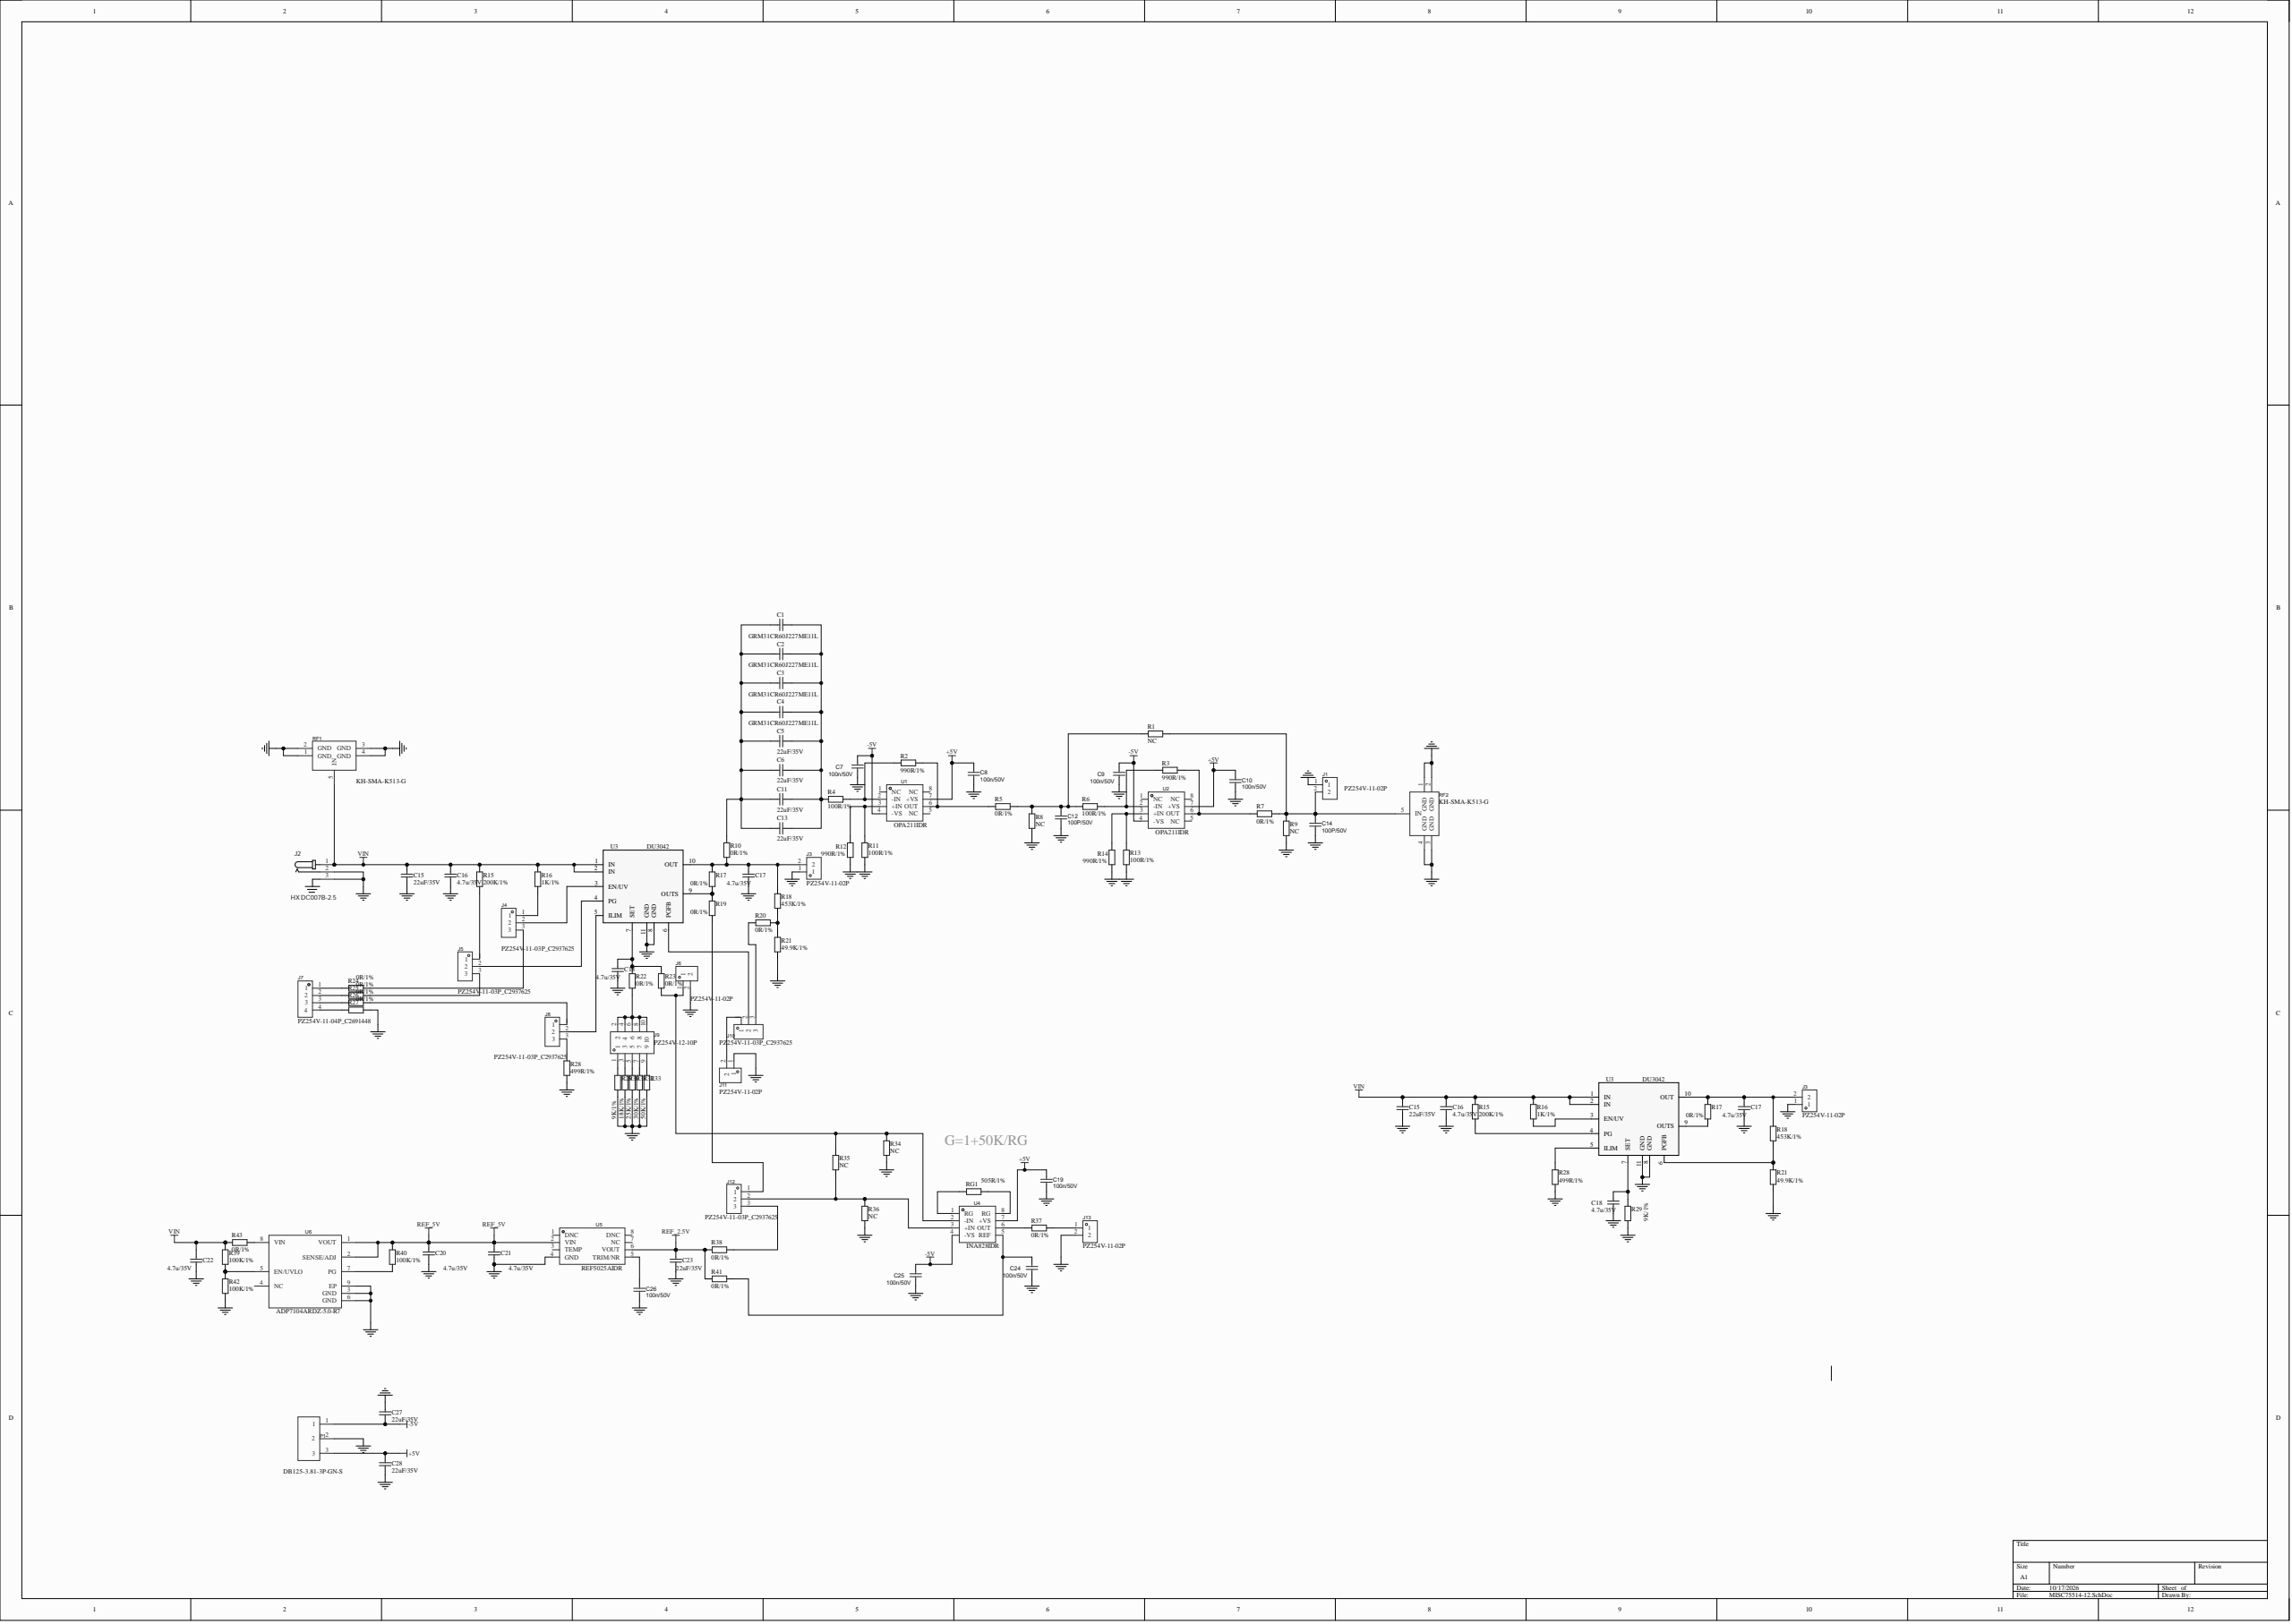Circuit board | Altium Designer | 107 parts | 62 nets
Bill of materials:
Comment,Description,Designator,Footprint,LibRef,Quantity
"GRM31CR60J227ME11L","SMD capacitor","C1, C2, C3, C4","C1206","C","4"
"22uF/35V","SMD capacitor","C5, C6, C11, C13, C15, C23, C27, C28","C1206","C","9"
"100n/50V","","C7, C8, C9, C10, C19, C24, C25, C26","C0603","1uF","8"
"100P/50V","","C12, C14","C0603","1uF","2"
"4.7u/35V","SMD capacitor","C16, C17, C18, C20, C21, C22","C0805","C","9"
"PZ254V-11-02P","","J1, J3, J6, J11, J13","HDR-TH_2P-P2.54-V-M","PZ254V-11-02P","6"
"HX DC007B-2.5","","J2","DC-IN-TH_HX-DC007B-2.5","HX DC007B-2.5","1"
"PZ254V-11-03P_C2937625","","J4, J5, J8, J10, J12","HDR-TH_3P-P2.54-V-M","PZ254V-11-03P_C2937625","5"
"PZ254V-11-04P_C2691448","","J7","HDR-TH_4P-P2.54-V-M","PZ254V-11-04P_C2691448","1"
"PZ254V-12-10P","","J9","HDR-TH_10P-P2.54-V-M-R2-C5-S2.54","PZ254V-12-10P","1"
"DB125-3.81-3P-GN-S","","P1","CONN-TH_3P-P3.81_L7.4-W11.4","WJ124-3.81-3P","1"
"NC","SMD resistor","R1, R8, R9, R34, R35, R36","R0603","R","6"
"990R/1%","SMD resistor","R2, R3, R12, R14","R0603","R","4"
"100R/1%","SMD resistor","R4, R6, R11, R13","R0603","R","4"
"0R/1%","SMD resistor","R5, R7, R10, R17, R19, R20, R22, R23, R24, R25, R26, R27, R37, R38, R41, R43","R0603","R","17"
"200K/1%","SMD resistor","R15","R0603","R","2"
"1K/1%","SMD resistor","R16","R0603","R","2"
"453K/1%","SMD resistor","R18","R0603","R","2"
"49.9K/1%","SMD resistor","R21","R0603","R","2"
"499R/1%","SMD resistor","R28","R0603","R","2"
"9K/1%","SMD resistor","R29","R0603","R","2"
"18K/1%","SMD resistor","R30","R0603","R","1"
"25K/1%","SMD resistor","R31","R0603","R","1"
"30K/1%","SMD resistor","R32","R0603","R","1"
"50K/1%","SMD resistor","R33","R0603","R","1"
"100K/1%","SMD resistor","R39, R40, R42","R0603","R","3"
"KH-SMA-K513-G","","RF1, RF2","ANT-TH_KH-SMA-K513-G","KH-SMA-K513-G","2"
"505R/1%","SMD resistor","RG1","R0603","R","1"
"OPA211IDR","","U1, U2","SOIC-8_L5.0-W4.0-P1.27-LS6.0-BL","INA828IDR","2"
"DU3042","No Description Available","U3","WSON-10_L3.0-W3.0-P0.50-BL-EP","DAC53202RTER","2"
"INA828IDR","","U4","SOIC-8_L5.0-W4.0-P1.27-LS6.0-BL","INA828IDR","1"
"REF5025AIDR","","U5","SOIC-8_L5.0-W4.0-P1.27-LS6.0-BL","REF5025AIDR","1"
"ADP7104ARDZ-5.0-R7","","U6","SOIC-8_L4.9-W3.9-P1.27-LS6.0-BL-EP","ADP7104ARDZ-5.0-R7","1"
Netlist (Protel format):
[
C1
C1206
GRM31CR60J227ME11L



]
[
C2
C1206
GRM31CR60J227ME11L



]
[
C3
C1206
GRM31CR60J227ME11L



]
[
C4
C1206
GRM31CR60J227ME11L



]
[
C5
C1206
22uF/35V



]
[
C6
C1206
22uF/35V



]
[
C7
C0603
100n/50V



]
[
C8
C0603
100n/50V



]
[
C9
C0603
100n/50V



]
[
C10
C0603
100n/50V



]
[
C11
C1206
22uF/35V



]
[
C12
C0603
100P/50V



]
[
C13
C1206
22uF/35V



]
[
C14
C0603
100P/50V



]
[
C15
C1206
22uF/35V



]
[
C15
C1206
22uF/35V



]
[
C16
C0805
4.7u/35V



]
[
C16
C0805
4.7u/35V



]
[
C17
C0805
4.7u/35V



]
[
C17
C0805
4.7u/35V



]
[
C18
C0805
4.7u/35V



]
[
C18
C0805
4.7u/35V



]
[
C19
C0603
100n/50V



]
[
C20
C0805
4.7u/35V



]
[
C21
C0805
4.7u/35V



]
[
C22
C0805
4.7u/35V



]
[
C23
C1206
22uF/35V



]
[
C24
C0603
100n/50V



]
[
C25
C0603
100n/50V



]
[
C26
C0603
100n/50V



]
[
C27
C1206
22uF/35V



]
[
C28
C1206
22uF/35V



]
[
J1
HDR-TH_2P-P2.54-V-M
PZ254V-11-02P



]
[
J2
DC-IN-TH_HX-DC007B-2.5
HX DC007B-2.5



]
[
J3
HDR-TH_2P-P2.54-V-M
PZ254V-11-02P



]
[
J3
HDR-TH_2P-P2.54-V-M
PZ254V-11-02P



]
[
J4
HDR-TH_3P-P2.54-V-M
PZ254V-11-03P_C2937625



]
[
J5
HDR-TH_3P-P2.54-V-M
PZ254V-11-03P_C2937625



]
[
J6
HDR-TH_2P-P2.54-V-M
PZ254V-11-02P



]
[
J7
HDR-TH_4P-P2.54-V-M
PZ254V-11-04P_C2691448



]
[
J8
HDR-TH_3P-P2.54-V-M
PZ254V-11-03P_C2937625



]
[
J9
HDR-TH_10P-P2.54-V-M-R2-C5-S2.54
PZ254V-12-10P



]
[
J10
HDR-TH_3P-P2.54-V-M
PZ254V-11-03P_C2937625



]
[
J11
HDR-TH_2P-P2.54-V-M
PZ254V-11-02P



]
[
J12
HDR-TH_3P-P2.54-V-M
PZ254V-11-03P_C2937625



]
[
J13
HDR-TH_2P-P2.54-V-M
PZ254V-11-02P



]
[
P1
CONN-TH_3P-P3.81_L7.4-W11.4
DB125-3.81-3P-GN-S



]
[
R1
R0603
NC



]
[
R2
R0603
990R/1%



]
[
R3
R0603
990R/1%



]
[
R4
R0603
100R/1%



]
[
R5
R0603
0R/1%



]
[
R6
R0603
100R/1%



]
[
R7
R0603
0R/1%



]
[
R8
R0603
NC



]
[
R9
R0603
NC



]
[
R10
R0603
0R/1%



]
[
R11
R0603
100R/1%



]
[
R12
R0603
990R/1%



]
[
R13
R0603
100R/1%



]
[
R14
R0603
990R/1%



]
[
R15
R0603
200K/1%



]
[
R15
R0603
200K/1%



]
[
R16
R0603
1K/1%



]
[
R16
R0603
1K/1%



]
[
R17
R0603
0R/1%



]
[
R17
R0603
0R/1%



]
[
R18
R0603
453K/1%



]
[
R18
R0603
453K/1%



]
[
R19
R0603
0R/1%



]
[
R20
R0603
0R/1%



]
[
R21
R0603
49.9K/1%



]
[
R21
R0603
49.9K/1%



]
[
R22
R0603
0R/1%



]
[
R23
R0603
0R/1%



]
[
R24
R0603
0R/1%



]
[
R25
R0603
0R/1%



]
[
R26
R0603
0R/1%



]
[
R27
R0603
0R/1%



]
[
R28
R0603
499R/1%



]
[
R28
R0603
499R/1%



]
[
R29
R0603
9K/1%



]
[
R29
R0603
9K/1%



]
[
R30
R0603
18K/1%



]
[
R31
R0603
25K/1%



]
[
R32
R0603
30K/1%



]
[
R33
R0603
50K/1%



]
[
R34
R0603
NC



]
[
R35
R0603
NC



]
[
R36
R0603
NC



]
[
R37
R0603
0R/1%



]
[
R38
R0603
0R/1%



]
[
R39
R0603
100K/1%



]
[
R40
R0603
100K/1%



]
[
R41
R0603
0R/1%



]
[
R42
R0603
100K/1%



]
[
R43
R0603
0R/1%



]
[
RF1
ANT-TH_KH-SMA-K513-G
KH-SMA-K513-G



]
[
RF2
ANT-TH_KH-SMA-K513-G
KH-SMA-K513-G



]
[
RG1
R0603
505R/1%



]
[
U1
SOIC-8_L5.0-W4.0-P1.27-LS6.0-BL
OPA211IDR



]
[
U2
SOIC-8_L5.0-W4.0-P1.27-LS6.0-BL
OPA211IDR



]
[
U3
WSON-10_L3.0-W3.0-P0.50-BL-EP
DU3042



]
[
U3
WSON-10_L3.0-W3.0-P0.50-BL-EP
DU3042



]
[
U4
SOIC-8_L5.0-W4.0-P1.27-LS6.0-BL
INA828IDR



]
[
U5
SOIC-8_L5.0-W4.0-P1.27-LS6.0-BL
REF5025AIDR



]
[
U6
SOIC-8_L4.9-W3.9-P1.27-LS6.0-BL-EP
ADP7104ARDZ-5.0-R7



]
(
VIN
C15-2
C15-2
C16-2
C16-2
C22-2
J2-1
R15-2
R15-2
R16-2
R16-2
R39-2
R43-1
RF1-5
U3-1
U3-1
U3-2
U3-2
)
(
REF_5V
C20-2
C21-2
R40-2
U5-2
U6-1
U6-2
)
(
REF_2.5V
C23-1
R38-1
R41-1
U5-6
)
(
NetRG1_2
RG1-2
U4-1
)
(
NetRG1_1
RG1-1
U4-8
)
(
NetR43_2
R43-2
U6-8
)
(
NetR40_1
R40-1
U6-7
)
(
NetR39_1
R39-1
R42-2
U6-5
)
(
NetR37_1
R37-1
U4-6
)
(
NetR28_2
R28-2
U3-5
)
(
NetR18_2
R18-2
R20-2
R21-1
)
(
NetR18_2
R18-2
R21-1
U3-6
)
(
NetR17_2
R17-2
R19-1
U3-9
)
(
NetR17_2
R17-2
U3-9
)
(
NetR16_1
R16-1
U3-3
)
(
NetR15_1
R15-1
U3-4
)
(
NetR13_2
R13-2
R14-2
U2-3
)
(
NetR11_2
R11-2
R12-2
U1-3
)
(
NetR3_2
R3-2
R6-2
U2-2
)
(
NetR3_1
R3-1
R7-1
U2-6
)
(
NetR2_2
R2-2
R4-2
U1-2
)
(
NetR2_1
R2-1
R5-1
U1-6
)
(
NetJ13_1
J13-1
R37-2
)
(
NetJ12_3
J12-3
R38-2
)
(
NetJ12_2
J12-2
R35-2
R36-1
U4-3
)
(
NetJ12_1
J12-1
R19-2
)
(
NetJ10_3
J10-3
R20-1
)
(
NetJ10_2
J10-2
U3-6
)
(
NetJ10_1
J10-1
J11-2
)
(
NetJ9_9
J9-9
R33-2
)
(
NetJ9_7
J9-7
R32-2
)
(
NetJ9_5
J9-5
R31-2
)
(
NetJ9_3
J9-3
R30-2
)
(
NetJ9_2
J9-2
J9-4
J9-6
J9-8
J9-10
R22-2
)
(
NetJ9_1
J9-1
R29-2
)
(
NetJ8_3
J8-3
R28-2
)
(
NetJ8_2
J8-2
U3-5
)
(
NetJ8_1
J8-1
R26-1
)
(
NetJ7_4
J7-4
R27-2
)
(
NetJ7_3
J7-3
R26-2
)
(
NetJ7_2
J7-2
R25-2
)
(
NetJ7_1
J7-1
R24-2
)
(
NetJ6_1
J6-1
R23-2
R34-1
R35-1
U4-2
)
(
NetJ5_3
J5-3
R25-1
)
(
NetJ5_2
J5-2
U3-4
)
(
NetJ5_1
J5-1
R15-1
)
(
NetJ4_3
J4-3
R24-1
)
(
NetJ4_2
J4-2
U3-3
)
(
NetJ4_1
J4-1
R16-1
)
(
NetC26_1
C26-1
U5-5
)
(
NetC24_1
C24-1
R41-2
U4-5
)
(
NetC18_2
C18-2
R22-1
R23-1
U3-7
)
(
NetC18_2
C18-2
R29-2
U3-7
)
(
NetC17_2
C17-2
J3-2
R10-2
R17-1
R18-1
U3-10
)
(
NetC17_2
C17-2
J3-2
R17-1
R18-1
U3-10
)
(
NetC14_1
C14-1
J1-2
R1-1
R7-2
R9-2
RF2-5
)
(
NetC12_1
C12-1
R1-2
R5-2
R6-1
R8-2
)
(
NetC1_2
C1-2
C2-2
C3-2
C4-2
C5-2
C6-2
C11-2
C13-2
R10-1
)
(
NetC1_1
C1-1
C2-1
C3-1
C4-1
C5-1
C6-1
C11-1
C13-1
R4-1
)
(
GND
C7-2
C8-2
C9-2
C10-2
C12-2
C14-2
C15-1
C15-1
C16-1
C16-1
C17-1
C17-1
C18-1
C18-1
C19-2
C20-1
C21-1
C22-1
C23-2
C24-2
C25-2
C26-2
C27-1
C28-1
J1-1
J2-2
J2-3
J3-1
J3-1
J6-2
J11-1
J13-2
P1-2
R8-1
R9-1
R11-1
R12-1
R13-1
R14-1
R21-2
R21-2
R27-1
R28-1
R28-1
R29-1
R29-1
R30-1
R31-1
R32-1
R33-1
R34-2
R36-2
R42-1
RF1-1
RF1-2
RF1-3
RF1-4
RF2-1
RF2-2
RF2-3
RF2-4
U3-8
U3-8
U3-11
U3-11
U5-4
U6-3
U6-6
U6-9
)
(
-5V
C7-1
C9-1
C25-1
C27-2
P1-1
U1-4
U2-4
U4-4
)
(
+5V
C8-1
C10-1
C19-1
C28-2
P1-3
U1-7
U2-7
U4-7
)